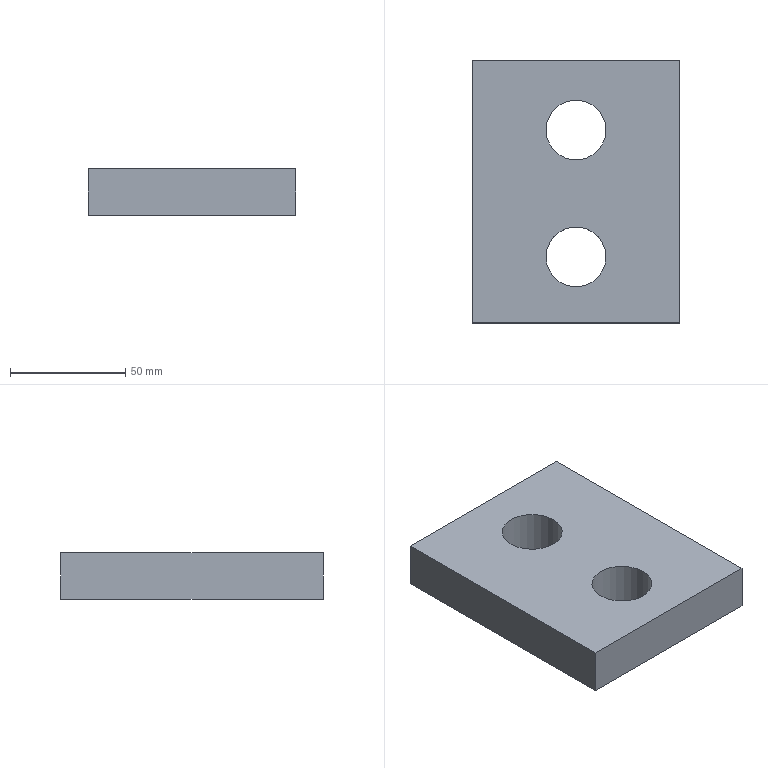Part | NX | features solid 2 | 1 solid | 8 faces | box 90 x 113.69 x 20 mm | volume 183404 mm3 | plane 6 | cylinder 2 | commonest cylinder face diameters 26 x2
STEP:
#1=CARTESIAN_POINT('',(332.5,-441.31,182.));
#2=VERTEX_POINT('',#1);
#3=CARTESIAN_POINT('',(345.5,-441.31,182.));
#4=DIRECTION('',(0.,0.,-1.));
#5=DIRECTION('',(-1.,0.,0.));
#6=AXIS2_PLACEMENT_3D('',#3,#4,#5);
#7=CIRCLE('',#6,13.);
#8=EDGE_CURVE('',#2,#2,#7,.T.);
#9=ORIENTED_EDGE('',*,*,#8,.F.);
#10=EDGE_LOOP('',(#9));
#11=FACE_BOUND('',#10,.T.);
#12=CARTESIAN_POINT('',(332.5,-386.31,182.));
#13=VERTEX_POINT('',#12);
#14=CARTESIAN_POINT('',(345.5,-386.31,182.));
#15=DIRECTION('',(0.,0.,-1.));
#16=DIRECTION('',(-1.,0.,0.));
#17=AXIS2_PLACEMENT_3D('',#14,#15,#16);
#18=CIRCLE('',#17,13.);
#19=EDGE_CURVE('',#13,#13,#18,.T.);
#20=ORIENTED_EDGE('',*,*,#19,.F.);
#21=EDGE_LOOP('',(#20));
#22=FACE_BOUND('',#21,.T.);
#23=CARTESIAN_POINT('',(390.5,-470.,182.));
#24=VERTEX_POINT('',#23);
#25=CARTESIAN_POINT('',(300.5,-470.,182.));
#26=VERTEX_POINT('',#25);
#27=CARTESIAN_POINT('',(1185.5,-470.,182.));
#28=DIRECTION('',(1.,0.,0.));
#29=VECTOR('',#28,1000.);
#30=LINE('',#27,#29);
#31=EDGE_CURVE('',#24,#26,#30,.F.);
#32=ORIENTED_EDGE('',*,*,#31,.T.);
#33=CARTESIAN_POINT('',(300.5,-356.31,182.));
#34=VERTEX_POINT('',#33);
#35=CARTESIAN_POINT('',(300.5,0.,182.));
#36=DIRECTION('',(0.,-1.,0.));
#37=VECTOR('',#36,1000.);
#38=LINE('',#35,#37);
#39=EDGE_CURVE('',#26,#34,#38,.F.);
#40=ORIENTED_EDGE('',*,*,#39,.T.);
#41=CARTESIAN_POINT('',(390.5,-356.31,182.));
#42=VERTEX_POINT('',#41);
#43=CARTESIAN_POINT('',(300.5,-356.31,182.));
#44=DIRECTION('',(-1.,0.,0.));
#45=VECTOR('',#44,1000.);
#46=LINE('',#43,#45);
#47=EDGE_CURVE('',#34,#42,#46,.F.);
#48=ORIENTED_EDGE('',*,*,#47,.T.);
#49=CARTESIAN_POINT('',(390.5,-346.31,182.));
#50=DIRECTION('',(0.,-1.,0.));
#51=VECTOR('',#50,1000.);
#52=LINE('',#49,#51);
#53=EDGE_CURVE('',#42,#24,#52,.T.);
#54=ORIENTED_EDGE('',*,*,#53,.T.);
#55=EDGE_LOOP('',(#32,#40,#48,#54));
#56=FACE_BOUND('',#55,.T.);
#57=CARTESIAN_POINT('',(399.5,-348.497,182.));
#58=DIRECTION('',(0.,0.,1.));
#59=DIRECTION('',(-1.,0.,0.));
#60=AXIS2_PLACEMENT_3D('',#57,#58,#59);
#61=PLANE('',#60);
#62=ADVANCED_FACE('',(#11,#22,#56),#61,.F.);
#63=CARTESIAN_POINT('',(390.5,-470.,202.));
#64=VERTEX_POINT('',#63);
#65=CARTESIAN_POINT('',(390.5,-470.,167.));
#66=DIRECTION('',(0.,0.,1.));
#67=VECTOR('',#66,1000.);
#68=LINE('',#65,#67);
#69=EDGE_CURVE('',#64,#24,#68,.F.);
#70=ORIENTED_EDGE('',*,*,#69,.F.);
#71=CARTESIAN_POINT('',(300.5,-470.,202.));
#72=VERTEX_POINT('',#71);
#73=CARTESIAN_POINT('',(1185.5,-470.,202.));
#74=DIRECTION('',(1.,0.,0.));
#75=VECTOR('',#74,1000.);
#76=LINE('',#73,#75);
#77=EDGE_CURVE('',#72,#64,#76,.T.);
#78=ORIENTED_EDGE('',*,*,#77,.F.);
#79=CARTESIAN_POINT('',(300.5,-470.,-68.));
#80=DIRECTION('',(0.,0.,-1.));
#81=VECTOR('',#80,1000.);
#82=LINE('',#79,#81);
#83=EDGE_CURVE('',#72,#26,#82,.T.);
#84=ORIENTED_EDGE('',*,*,#83,.T.);
#85=ORIENTED_EDGE('',*,*,#31,.F.);
#86=EDGE_LOOP('',(#70,#78,#84,#85));
#87=FACE_BOUND('',#86,.T.);
#88=CARTESIAN_POINT('',(1185.5,-470.,167.));
#89=DIRECTION('',(0.,-1.,0.));
#90=DIRECTION('',(0.,0.,-1.));
#91=AXIS2_PLACEMENT_3D('',#88,#89,#90);
#92=PLANE('',#91);
#93=ADVANCED_FACE('',(#87),#92,.T.);
#94=ORIENTED_EDGE('',*,*,#83,.F.);
#95=CARTESIAN_POINT('',(300.5,-356.31,202.));
#96=VERTEX_POINT('',#95);
#97=CARTESIAN_POINT('',(300.5,0.,202.));
#98=DIRECTION('',(0.,-1.,0.));
#99=VECTOR('',#98,1000.);
#100=LINE('',#97,#99);
#101=EDGE_CURVE('',#96,#72,#100,.T.);
#102=ORIENTED_EDGE('',*,*,#101,.F.);
#103=CARTESIAN_POINT('',(300.5,-356.31,-3.));
#104=DIRECTION('',(0.,0.,-1.));
#105=VECTOR('',#104,1000.);
#106=LINE('',#103,#105);
#107=EDGE_CURVE('',#96,#34,#106,.T.);
#108=ORIENTED_EDGE('',*,*,#107,.T.);
#109=ORIENTED_EDGE('',*,*,#39,.F.);
#110=EDGE_LOOP('',(#94,#102,#108,#109));
#111=FACE_BOUND('',#110,.T.);
#112=CARTESIAN_POINT('',(300.5,0.,-68.));
#113=DIRECTION('',(-1.,0.,0.));
#114=DIRECTION('',(0.,0.,-1.));
#115=AXIS2_PLACEMENT_3D('',#112,#113,#114);
#116=PLANE('',#115);
#117=ADVANCED_FACE('',(#111),#116,.T.);
#118=ORIENTED_EDGE('',*,*,#107,.F.);
#119=CARTESIAN_POINT('',(390.5,-356.31,202.));
#120=VERTEX_POINT('',#119);
#121=CARTESIAN_POINT('',(300.5,-356.31,202.));
#122=DIRECTION('',(-1.,0.,0.));
#123=VECTOR('',#122,1000.);
#124=LINE('',#121,#123);
#125=EDGE_CURVE('',#120,#96,#124,.T.);
#126=ORIENTED_EDGE('',*,*,#125,.F.);
#127=CARTESIAN_POINT('',(390.5,-356.31,187.));
#128=DIRECTION('',(0.,0.,1.));
#129=VECTOR('',#128,1000.);
#130=LINE('',#127,#129);
#131=EDGE_CURVE('',#120,#42,#130,.F.);
#132=ORIENTED_EDGE('',*,*,#131,.T.);
#133=ORIENTED_EDGE('',*,*,#47,.F.);
#134=EDGE_LOOP('',(#118,#126,#132,#133));
#135=FACE_BOUND('',#134,.T.);
#136=CARTESIAN_POINT('',(300.5,-356.31,-3.));
#137=DIRECTION('',(0.,1.,0.));
#138=DIRECTION('',(0.,0.,-1.));
#139=AXIS2_PLACEMENT_3D('',#136,#137,#138);
#140=PLANE('',#139);
#141=ADVANCED_FACE('',(#135),#140,.T.);
#142=CARTESIAN_POINT('',(332.5,-441.31,202.));
#143=VERTEX_POINT('',#142);
#144=CARTESIAN_POINT('',(345.5,-441.31,202.));
#145=DIRECTION('',(0.,0.,-1.));
#146=DIRECTION('',(-1.,0.,0.));
#147=AXIS2_PLACEMENT_3D('',#144,#145,#146);
#148=CIRCLE('',#147,13.);
#149=EDGE_CURVE('',#143,#143,#148,.T.);
#150=ORIENTED_EDGE('',*,*,#149,.T.);
#151=EDGE_LOOP('',(#150));
#152=FACE_BOUND('',#151,.T.);
#153=CARTESIAN_POINT('',(332.5,-386.31,202.));
#154=VERTEX_POINT('',#153);
#155=CARTESIAN_POINT('',(345.5,-386.31,202.));
#156=DIRECTION('',(0.,0.,-1.));
#157=DIRECTION('',(-1.,0.,0.));
#158=AXIS2_PLACEMENT_3D('',#155,#156,#157);
#159=CIRCLE('',#158,13.);
#160=EDGE_CURVE('',#154,#154,#159,.T.);
#161=ORIENTED_EDGE('',*,*,#160,.T.);
#162=EDGE_LOOP('',(#161));
#163=FACE_BOUND('',#162,.T.);
#164=CARTESIAN_POINT('',(390.5,-346.31,202.));
#165=DIRECTION('',(0.,-1.,0.));
#166=VECTOR('',#165,1000.);
#167=LINE('',#164,#166);
#168=EDGE_CURVE('',#64,#120,#167,.F.);
#169=ORIENTED_EDGE('',*,*,#168,.T.);
#170=ORIENTED_EDGE('',*,*,#125,.T.);
#171=ORIENTED_EDGE('',*,*,#101,.T.);
#172=ORIENTED_EDGE('',*,*,#77,.T.);
#173=EDGE_LOOP('',(#169,#170,#171,#172));
#174=FACE_BOUND('',#173,.T.);
#175=CARTESIAN_POINT('',(345.5,-414.249,202.));
#176=DIRECTION('',(0.,0.,1.));
#177=DIRECTION('',(-1.,0.,0.));
#178=AXIS2_PLACEMENT_3D('',#175,#176,#177);
#179=PLANE('',#178);
#180=ADVANCED_FACE('',(#152,#163,#174),#179,.T.);
#181=ORIENTED_EDGE('',*,*,#168,.F.);
#182=ORIENTED_EDGE('',*,*,#69,.T.);
#183=ORIENTED_EDGE('',*,*,#53,.F.);
#184=ORIENTED_EDGE('',*,*,#131,.F.);
#185=EDGE_LOOP('',(#181,#182,#183,#184));
#186=FACE_BOUND('',#185,.T.);
#187=CARTESIAN_POINT('',(390.5,-346.31,187.));
#188=DIRECTION('',(-1.,0.,0.));
#189=DIRECTION('',(0.,0.,-1.));
#190=AXIS2_PLACEMENT_3D('',#187,#188,#189);
#191=PLANE('',#190);
#192=ADVANCED_FACE('',(#186),#191,.F.);
#193=ORIENTED_EDGE('',*,*,#160,.F.);
#194=EDGE_LOOP('',(#193));
#195=FACE_BOUND('',#194,.T.);
#196=ORIENTED_EDGE('',*,*,#19,.T.);
#197=EDGE_LOOP('',(#196));
#198=FACE_BOUND('',#197,.T.);
#199=CARTESIAN_POINT('',(345.5,-386.31,182.));
#200=DIRECTION('',(0.,0.,1.));
#201=DIRECTION('',(-1.,0.,0.));
#202=AXIS2_PLACEMENT_3D('',#199,#200,#201);
#203=CYLINDRICAL_SURFACE('',#202,13.);
#204=ADVANCED_FACE('',(#195,#198),#203,.F.);
#205=ORIENTED_EDGE('',*,*,#149,.F.);
#206=EDGE_LOOP('',(#205));
#207=FACE_BOUND('',#206,.T.);
#208=ORIENTED_EDGE('',*,*,#8,.T.);
#209=EDGE_LOOP('',(#208));
#210=FACE_BOUND('',#209,.T.);
#211=CARTESIAN_POINT('',(345.5,-441.31,182.));
#212=DIRECTION('',(0.,0.,1.));
#213=DIRECTION('',(-1.,0.,0.));
#214=AXIS2_PLACEMENT_3D('',#211,#212,#213);
#215=CYLINDRICAL_SURFACE('',#214,13.);
#216=ADVANCED_FACE('',(#207,#210),#215,.F.);
#217=CLOSED_SHELL('',(#62,#93,#117,#141,#180,#192,#204,#216));
#218=MANIFOLD_SOLID_BREP('',#217);
#219=(LENGTH_UNIT()NAMED_UNIT(*)SI_UNIT(.MILLI.,.METRE.));
#220=UNCERTAINTY_MEASURE_WITH_UNIT(LENGTH_MEASURE(0.00001),#219,'','');
#221=(NAMED_UNIT(*)PLANE_ANGLE_UNIT()SI_UNIT($,.RADIAN.));
#222=(NAMED_UNIT(*)SI_UNIT($,.STERADIAN.)SOLID_ANGLE_UNIT());
#223=(GEOMETRIC_REPRESENTATION_CONTEXT(3)GLOBAL_UNCERTAINTY_ASSIGNED_CONTEXT((#220))GLOBAL_UNIT_ASSIGNED_CONTEXT((#219,#221,#222))REPRESENTATION_CONTEXT('',''));
#224=ADVANCED_BREP_SHAPE_REPRESENTATION('',(#218),#223);